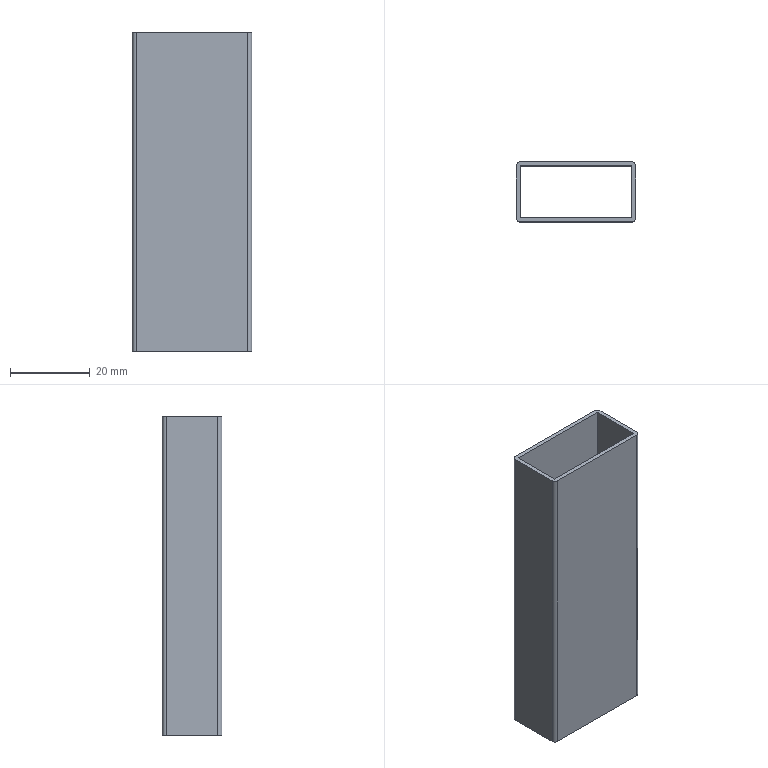Part | STEP file | Q7C1211 | 1 solid | 14 faces | box 30 x 15 x 80 mm | volume 6811 mm3 | plane 10 | cylinder 4 | commonest cylinder face diameters 2 x4
STEP:
#1=CARTESIAN_POINT('',(0.,0.,0.));
#2=DIRECTION('',(0.,0.,1.));
#3=DIRECTION('',(1.,0.,0.));
#4=AXIS2_PLACEMENT_3D('',#1,#2,#3);
#5=CARTESIAN_POINT('',(15.,6.5,40.));
#6=VERTEX_POINT('',#5);
#7=CARTESIAN_POINT('',(14.,7.5,40.));
#8=VERTEX_POINT('',#7);
#9=CARTESIAN_POINT('',(14.,6.5,40.));
#10=DIRECTION('',(0.,0.,1.));
#11=DIRECTION('',(-1.,0.,0.));
#12=AXIS2_PLACEMENT_3D('',#9,#10,#11);
#13=CIRCLE('',#12,1.);
#14=CARTESIAN_POINT('',(14.,6.5,40.));
#15=DIRECTION('',(0.,0.,-1.));
#16=DIRECTION('',(-1.,0.,0.));
#17=AXIS2_PLACEMENT_3D('',#14,#15,#16);
#18=PLANE('',#17);
#19=CARTESIAN_POINT('',(1.,0.));
#20=CARTESIAN_POINT('',(1.,-1.732));
#21=CARTESIAN_POINT('',(-0.5,-0.866));
#22=CARTESIAN_POINT('',(-2.,0.));
#23=CARTESIAN_POINT('',(-0.5,0.866));
#24=CARTESIAN_POINT('',(1.,1.732));
#25=CARTESIAN_POINT('',(1.,0.));
#26=(BOUNDED_CURVE()B_SPLINE_CURVE(2,(#19,#20,#21,#22,#23,#24,#25),.UNSPECIFIED.,.T.,.F.)B_SPLINE_CURVE_WITH_KNOTS((1,2,2,2,2,1),(-2.094,0.,2.094,4.189,6.283,8.378),.UNSPECIFIED.)CURVE()GEOMETRIC_REPRESENTATION_ITEM()RATIONAL_B_SPLINE_CURVE((1.,0.5,1.,0.5,1.,0.5,1.))REPRESENTATION_ITEM(''));
#27=(GEOMETRIC_REPRESENTATION_CONTEXT(2)PARAMETRIC_REPRESENTATION_CONTEXT()REPRESENTATION_CONTEXT('',''));
#28=DEFINITIONAL_REPRESENTATION('',(#26),#27);
#29=PCURVE('',#18,#28);
#30=CARTESIAN_POINT('',(14.,6.5,40.));
#31=DIRECTION('',(0.,0.,-1.));
#32=DIRECTION('',(-1.,0.,0.));
#33=AXIS2_PLACEMENT_3D('',#30,#31,#32);
#34=CYLINDRICAL_SURFACE('',#33,1.);
#35=CARTESIAN_POINT('',(6.283,0.));
#36=DIRECTION('',(-1.,0.));
#37=VECTOR('',#36,1.);
#38=LINE('',#35,#37);
#39=(GEOMETRIC_REPRESENTATION_CONTEXT(2)PARAMETRIC_REPRESENTATION_CONTEXT()REPRESENTATION_CONTEXT('',''));
#40=DEFINITIONAL_REPRESENTATION('',(#38),#39);
#41=PCURVE('',#34,#40);
#42=SURFACE_CURVE('',#13,(#29,#41),.PCURVE_S1.);
#43=EDGE_CURVE('',#6,#8,#42,.T.);
#44=ORIENTED_EDGE('',*,*,#43,.T.);
#45=CARTESIAN_POINT('',(-14.,7.5,40.));
#46=VERTEX_POINT('',#45);
#47=CARTESIAN_POINT('',(-14.,7.5,40.));
#48=DIRECTION('',(-1.,0.,0.));
#49=VECTOR('',#48,1.);
#50=LINE('',#47,#49);
#51=CARTESIAN_POINT('',(28.,1.));
#52=DIRECTION('',(1.,0.));
#53=VECTOR('',#52,1.);
#54=LINE('',#51,#53);
#55=(GEOMETRIC_REPRESENTATION_CONTEXT(2)PARAMETRIC_REPRESENTATION_CONTEXT()REPRESENTATION_CONTEXT('',''));
#56=DEFINITIONAL_REPRESENTATION('',(#54),#55);
#57=PCURVE('',#18,#56);
#58=CARTESIAN_POINT('',(-14.,7.5,40.));
#59=DIRECTION('',(0.,-1.,0.));
#60=DIRECTION('',(0.,0.,-1.));
#61=AXIS2_PLACEMENT_3D('',#58,#59,#60);
#62=PLANE('',#61);
#63=CARTESIAN_POINT('',(0.,0.));
#64=DIRECTION('',(0.,-1.));
#65=VECTOR('',#64,1.);
#66=LINE('',#63,#65);
#67=(GEOMETRIC_REPRESENTATION_CONTEXT(2)PARAMETRIC_REPRESENTATION_CONTEXT()REPRESENTATION_CONTEXT('',''));
#68=DEFINITIONAL_REPRESENTATION('',(#66),#67);
#69=PCURVE('',#62,#68);
#70=SURFACE_CURVE('',#50,(#57,#69),.PCURVE_S1.);
#71=EDGE_CURVE('',#8,#46,#70,.T.);
#72=ORIENTED_EDGE('',*,*,#71,.T.);
#73=CARTESIAN_POINT('',(-15.,6.5,40.));
#74=VERTEX_POINT('',#73);
#75=CARTESIAN_POINT('',(-14.,6.5,40.));
#76=DIRECTION('',(0.,0.,1.));
#77=DIRECTION('',(1.,0.,0.));
#78=AXIS2_PLACEMENT_3D('',#75,#76,#77);
#79=CIRCLE('',#78,1.);
#80=CARTESIAN_POINT('',(27.,0.));
#81=CARTESIAN_POINT('',(27.,1.732));
#82=CARTESIAN_POINT('',(28.5,0.866));
#83=CARTESIAN_POINT('',(30.,0.));
#84=CARTESIAN_POINT('',(28.5,-0.866));
#85=CARTESIAN_POINT('',(27.,-1.732));
#86=CARTESIAN_POINT('',(27.,0.));
#87=(BOUNDED_CURVE()B_SPLINE_CURVE(2,(#80,#81,#82,#83,#84,#85,#86),.UNSPECIFIED.,.T.,.F.)B_SPLINE_CURVE_WITH_KNOTS((1,2,2,2,2,1),(-2.094,0.,2.094,4.189,6.283,8.378),.UNSPECIFIED.)CURVE()GEOMETRIC_REPRESENTATION_ITEM()RATIONAL_B_SPLINE_CURVE((1.,0.5,1.,0.5,1.,0.5,1.))REPRESENTATION_ITEM(''));
#88=(GEOMETRIC_REPRESENTATION_CONTEXT(2)PARAMETRIC_REPRESENTATION_CONTEXT()REPRESENTATION_CONTEXT('',''));
#89=DEFINITIONAL_REPRESENTATION('',(#87),#88);
#90=PCURVE('',#18,#89);
#91=CARTESIAN_POINT('',(-14.,6.5,40.));
#92=DIRECTION('',(0.,0.,-1.));
#93=DIRECTION('',(-1.,0.,0.));
#94=AXIS2_PLACEMENT_3D('',#91,#92,#93);
#95=CYLINDRICAL_SURFACE('',#94,1.);
#96=CARTESIAN_POINT('',(3.142,0.));
#97=DIRECTION('',(-1.,0.));
#98=VECTOR('',#97,1.);
#99=LINE('',#96,#98);
#100=(GEOMETRIC_REPRESENTATION_CONTEXT(2)PARAMETRIC_REPRESENTATION_CONTEXT()REPRESENTATION_CONTEXT('',''));
#101=DEFINITIONAL_REPRESENTATION('',(#99),#100);
#102=PCURVE('',#95,#101);
#103=SURFACE_CURVE('',#79,(#90,#102),.PCURVE_S1.);
#104=EDGE_CURVE('',#46,#74,#103,.T.);
#105=ORIENTED_EDGE('',*,*,#104,.T.);
#106=CARTESIAN_POINT('',(-15.,-6.5,40.));
#107=VERTEX_POINT('',#106);
#108=CARTESIAN_POINT('',(-15.,6.5,40.));
#109=DIRECTION('',(0.,-1.,0.));
#110=VECTOR('',#109,1.);
#111=LINE('',#108,#110);
#112=CARTESIAN_POINT('',(29.,0.));
#113=DIRECTION('',(0.,-1.));
#114=VECTOR('',#113,1.);
#115=LINE('',#112,#114);
#116=(GEOMETRIC_REPRESENTATION_CONTEXT(2)PARAMETRIC_REPRESENTATION_CONTEXT()REPRESENTATION_CONTEXT('',''));
#117=DEFINITIONAL_REPRESENTATION('',(#115),#116);
#118=PCURVE('',#18,#117);
#119=CARTESIAN_POINT('',(-15.,6.5,40.));
#120=DIRECTION('',(1.,0.,0.));
#121=DIRECTION('',(0.,1.,0.));
#122=AXIS2_PLACEMENT_3D('',#119,#120,#121);
#123=PLANE('',#122);
#124=CARTESIAN_POINT('',(0.,0.));
#125=DIRECTION('',(-1.,0.));
#126=VECTOR('',#125,1.);
#127=LINE('',#124,#126);
#128=(GEOMETRIC_REPRESENTATION_CONTEXT(2)PARAMETRIC_REPRESENTATION_CONTEXT()REPRESENTATION_CONTEXT('',''));
#129=DEFINITIONAL_REPRESENTATION('',(#127),#128);
#130=PCURVE('',#123,#129);
#131=SURFACE_CURVE('',#111,(#118,#130),.PCURVE_S1.);
#132=EDGE_CURVE('',#74,#107,#131,.T.);
#133=ORIENTED_EDGE('',*,*,#132,.T.);
#134=CARTESIAN_POINT('',(-14.,-7.5,40.));
#135=VERTEX_POINT('',#134);
#136=CARTESIAN_POINT('',(-14.,-6.5,40.));
#137=DIRECTION('',(0.,0.,1.));
#138=DIRECTION('',(1.,0.,0.));
#139=AXIS2_PLACEMENT_3D('',#136,#137,#138);
#140=CIRCLE('',#139,1.);
#141=CARTESIAN_POINT('',(27.,-13.));
#142=CARTESIAN_POINT('',(27.,-11.268));
#143=CARTESIAN_POINT('',(28.5,-12.134));
#144=CARTESIAN_POINT('',(30.,-13.));
#145=CARTESIAN_POINT('',(28.5,-13.866));
#146=CARTESIAN_POINT('',(27.,-14.732));
#147=CARTESIAN_POINT('',(27.,-13.));
#148=(BOUNDED_CURVE()B_SPLINE_CURVE(2,(#141,#142,#143,#144,#145,#146,#147),.UNSPECIFIED.,.T.,.F.)B_SPLINE_CURVE_WITH_KNOTS((1,2,2,2,2,1),(-2.094,0.,2.094,4.189,6.283,8.378),.UNSPECIFIED.)CURVE()GEOMETRIC_REPRESENTATION_ITEM()RATIONAL_B_SPLINE_CURVE((1.,0.5,1.,0.5,1.,0.5,1.))REPRESENTATION_ITEM(''));
#149=(GEOMETRIC_REPRESENTATION_CONTEXT(2)PARAMETRIC_REPRESENTATION_CONTEXT()REPRESENTATION_CONTEXT('',''));
#150=DEFINITIONAL_REPRESENTATION('',(#148),#149);
#151=PCURVE('',#18,#150);
#152=CARTESIAN_POINT('',(-14.,-6.5,40.));
#153=DIRECTION('',(0.,0.,-1.));
#154=DIRECTION('',(-1.,0.,0.));
#155=AXIS2_PLACEMENT_3D('',#152,#153,#154);
#156=CYLINDRICAL_SURFACE('',#155,1.);
#157=CARTESIAN_POINT('',(9.425,0.));
#158=DIRECTION('',(-1.,0.));
#159=VECTOR('',#158,1.);
#160=LINE('',#157,#159);
#161=(GEOMETRIC_REPRESENTATION_CONTEXT(2)PARAMETRIC_REPRESENTATION_CONTEXT()REPRESENTATION_CONTEXT('',''));
#162=DEFINITIONAL_REPRESENTATION('',(#160),#161);
#163=PCURVE('',#156,#162);
#164=SURFACE_CURVE('',#140,(#151,#163),.PCURVE_S1.);
#165=EDGE_CURVE('',#107,#135,#164,.T.);
#166=ORIENTED_EDGE('',*,*,#165,.T.);
#167=CARTESIAN_POINT('',(14.,-7.5,40.));
#168=VERTEX_POINT('',#167);
#169=CARTESIAN_POINT('',(-14.,-7.5,40.));
#170=DIRECTION('',(1.,0.,0.));
#171=VECTOR('',#170,1.);
#172=LINE('',#169,#171);
#173=CARTESIAN_POINT('',(28.,-14.));
#174=DIRECTION('',(-1.,0.));
#175=VECTOR('',#174,1.);
#176=LINE('',#173,#175);
#177=(GEOMETRIC_REPRESENTATION_CONTEXT(2)PARAMETRIC_REPRESENTATION_CONTEXT()REPRESENTATION_CONTEXT('',''));
#178=DEFINITIONAL_REPRESENTATION('',(#176),#177);
#179=PCURVE('',#18,#178);
#180=CARTESIAN_POINT('',(-14.,-7.5,40.));
#181=DIRECTION('',(0.,1.,0.));
#182=DIRECTION('',(0.,0.,1.));
#183=AXIS2_PLACEMENT_3D('',#180,#181,#182);
#184=PLANE('',#183);
#185=CARTESIAN_POINT('',(0.,0.));
#186=DIRECTION('',(0.,1.));
#187=VECTOR('',#186,1.);
#188=LINE('',#185,#187);
#189=(GEOMETRIC_REPRESENTATION_CONTEXT(2)PARAMETRIC_REPRESENTATION_CONTEXT()REPRESENTATION_CONTEXT('',''));
#190=DEFINITIONAL_REPRESENTATION('',(#188),#189);
#191=PCURVE('',#184,#190);
#192=SURFACE_CURVE('',#172,(#179,#191),.PCURVE_S1.);
#193=EDGE_CURVE('',#135,#168,#192,.T.);
#194=ORIENTED_EDGE('',*,*,#193,.T.);
#195=CARTESIAN_POINT('',(15.,-6.5,40.));
#196=VERTEX_POINT('',#195);
#197=CARTESIAN_POINT('',(14.,-6.5,40.));
#198=DIRECTION('',(0.,0.,1.));
#199=DIRECTION('',(1.,0.,0.));
#200=AXIS2_PLACEMENT_3D('',#197,#198,#199);
#201=CIRCLE('',#200,1.);
#202=CARTESIAN_POINT('',(-1.,-13.));
#203=CARTESIAN_POINT('',(-1.,-11.268));
#204=CARTESIAN_POINT('',(0.5,-12.134));
#205=CARTESIAN_POINT('',(2.,-13.));
#206=CARTESIAN_POINT('',(0.5,-13.866));
#207=CARTESIAN_POINT('',(-1.,-14.732));
#208=CARTESIAN_POINT('',(-1.,-13.));
#209=(BOUNDED_CURVE()B_SPLINE_CURVE(2,(#202,#203,#204,#205,#206,#207,#208),.UNSPECIFIED.,.T.,.F.)B_SPLINE_CURVE_WITH_KNOTS((1,2,2,2,2,1),(-2.094,0.,2.094,4.189,6.283,8.378),.UNSPECIFIED.)CURVE()GEOMETRIC_REPRESENTATION_ITEM()RATIONAL_B_SPLINE_CURVE((1.,0.5,1.,0.5,1.,0.5,1.))REPRESENTATION_ITEM(''));
#210=(GEOMETRIC_REPRESENTATION_CONTEXT(2)PARAMETRIC_REPRESENTATION_CONTEXT()REPRESENTATION_CONTEXT('',''));
#211=DEFINITIONAL_REPRESENTATION('',(#209),#210);
#212=PCURVE('',#18,#211);
#213=CARTESIAN_POINT('',(14.,-6.5,40.));
#214=DIRECTION('',(0.,0.,-1.));
#215=DIRECTION('',(-1.,0.,0.));
#216=AXIS2_PLACEMENT_3D('',#213,#214,#215);
#217=CYLINDRICAL_SURFACE('',#216,1.);
#218=CARTESIAN_POINT('',(9.425,0.));
#219=DIRECTION('',(-1.,0.));
#220=VECTOR('',#219,1.);
#221=LINE('',#218,#220);
#222=(GEOMETRIC_REPRESENTATION_CONTEXT(2)PARAMETRIC_REPRESENTATION_CONTEXT()REPRESENTATION_CONTEXT('',''));
#223=DEFINITIONAL_REPRESENTATION('',(#221),#222);
#224=PCURVE('',#217,#223);
#225=SURFACE_CURVE('',#201,(#212,#224),.PCURVE_S1.);
#226=EDGE_CURVE('',#168,#196,#225,.T.);
#227=ORIENTED_EDGE('',*,*,#226,.T.);
#228=CARTESIAN_POINT('',(15.,6.5,40.));
#229=DIRECTION('',(0.,1.,0.));
#230=VECTOR('',#229,1.);
#231=LINE('',#228,#230);
#232=CARTESIAN_POINT('',(-1.,0.));
#233=DIRECTION('',(0.,1.));
#234=VECTOR('',#233,1.);
#235=LINE('',#232,#234);
#236=(GEOMETRIC_REPRESENTATION_CONTEXT(2)PARAMETRIC_REPRESENTATION_CONTEXT()REPRESENTATION_CONTEXT('',''));
#237=DEFINITIONAL_REPRESENTATION('',(#235),#236);
#238=PCURVE('',#18,#237);
#239=CARTESIAN_POINT('',(15.,6.5,40.));
#240=DIRECTION('',(-1.,0.,0.));
#241=DIRECTION('',(0.,0.,1.));
#242=AXIS2_PLACEMENT_3D('',#239,#240,#241);
#243=PLANE('',#242);
#244=CARTESIAN_POINT('',(0.,0.));
#245=DIRECTION('',(0.,1.));
#246=VECTOR('',#245,1.);
#247=LINE('',#244,#246);
#248=(GEOMETRIC_REPRESENTATION_CONTEXT(2)PARAMETRIC_REPRESENTATION_CONTEXT()REPRESENTATION_CONTEXT('',''));
#249=DEFINITIONAL_REPRESENTATION('',(#247),#248);
#250=PCURVE('',#243,#249);
#251=SURFACE_CURVE('',#231,(#238,#250),.PCURVE_S1.);
#252=EDGE_CURVE('',#196,#6,#251,.T.);
#253=ORIENTED_EDGE('',*,*,#252,.T.);
#254=EDGE_LOOP('',(#44,#72,#105,#133,#166,#194,#227,#253));
#255=FACE_BOUND('',#254,.T.);
#256=CARTESIAN_POINT('',(14.,6.5,40.));
#257=VERTEX_POINT('',#256);
#258=CARTESIAN_POINT('',(-14.,6.5,40.));
#259=VERTEX_POINT('',#258);
#260=CARTESIAN_POINT('',(-14.,6.5,40.));
#261=DIRECTION('',(-1.,0.,0.));
#262=VECTOR('',#261,1.);
#263=LINE('',#260,#262);
#264=CARTESIAN_POINT('',(28.,0.));
#265=DIRECTION('',(1.,0.));
#266=VECTOR('',#265,1.);
#267=LINE('',#264,#266);
#268=(GEOMETRIC_REPRESENTATION_CONTEXT(2)PARAMETRIC_REPRESENTATION_CONTEXT()REPRESENTATION_CONTEXT('',''));
#269=DEFINITIONAL_REPRESENTATION('',(#267),#268);
#270=PCURVE('',#18,#269);
#271=CARTESIAN_POINT('',(-14.,6.5,40.));
#272=DIRECTION('',(0.,-1.,0.));
#273=DIRECTION('',(0.,0.,-1.));
#274=AXIS2_PLACEMENT_3D('',#271,#272,#273);
#275=PLANE('',#274);
#276=CARTESIAN_POINT('',(0.,0.));
#277=DIRECTION('',(0.,-1.));
#278=VECTOR('',#277,1.);
#279=LINE('',#276,#278);
#280=(GEOMETRIC_REPRESENTATION_CONTEXT(2)PARAMETRIC_REPRESENTATION_CONTEXT()REPRESENTATION_CONTEXT('',''));
#281=DEFINITIONAL_REPRESENTATION('',(#279),#280);
#282=PCURVE('',#275,#281);
#283=SURFACE_CURVE('',#263,(#270,#282),.PCURVE_S1.);
#284=EDGE_CURVE('',#257,#259,#283,.T.);
#285=ORIENTED_EDGE('',*,*,#284,.F.);
#286=CARTESIAN_POINT('',(14.,-6.5,40.));
#287=VERTEX_POINT('',#286);
#288=CARTESIAN_POINT('',(14.,6.5,40.));
#289=DIRECTION('',(0.,1.,0.));
#290=VECTOR('',#289,1.);
#291=LINE('',#288,#290);
#292=CARTESIAN_POINT('',(0.,0.));
#293=DIRECTION('',(0.,1.));
#294=VECTOR('',#293,1.);
#295=LINE('',#292,#294);
#296=(GEOMETRIC_REPRESENTATION_CONTEXT(2)PARAMETRIC_REPRESENTATION_CONTEXT()REPRESENTATION_CONTEXT('',''));
#297=DEFINITIONAL_REPRESENTATION('',(#295),#296);
#298=PCURVE('',#18,#297);
#299=CARTESIAN_POINT('',(14.,6.5,40.));
#300=DIRECTION('',(-1.,0.,0.));
#301=DIRECTION('',(0.,-1.,0.));
#302=AXIS2_PLACEMENT_3D('',#299,#300,#301);
#303=PLANE('',#302);
#304=CARTESIAN_POINT('',(0.,0.));
#305=DIRECTION('',(-1.,0.));
#306=VECTOR('',#305,1.);
#307=LINE('',#304,#306);
#308=(GEOMETRIC_REPRESENTATION_CONTEXT(2)PARAMETRIC_REPRESENTATION_CONTEXT()REPRESENTATION_CONTEXT('',''));
#309=DEFINITIONAL_REPRESENTATION('',(#307),#308);
#310=PCURVE('',#303,#309);
#311=SURFACE_CURVE('',#291,(#298,#310),.PCURVE_S1.);
#312=EDGE_CURVE('',#287,#257,#311,.T.);
#313=ORIENTED_EDGE('',*,*,#312,.F.);
#314=CARTESIAN_POINT('',(-14.,-6.5,40.));
#315=VERTEX_POINT('',#314);
#316=CARTESIAN_POINT('',(-14.,-6.5,40.));
#317=DIRECTION('',(1.,0.,0.));
#318=VECTOR('',#317,1.);
#319=LINE('',#316,#318);
#320=CARTESIAN_POINT('',(28.,-13.));
#321=DIRECTION('',(-1.,0.));
#322=VECTOR('',#321,1.);
#323=LINE('',#320,#322);
#324=(GEOMETRIC_REPRESENTATION_CONTEXT(2)PARAMETRIC_REPRESENTATION_CONTEXT()REPRESENTATION_CONTEXT('',''));
#325=DEFINITIONAL_REPRESENTATION('',(#323),#324);
#326=PCURVE('',#18,#325);
#327=CARTESIAN_POINT('',(-14.,-6.5,40.));
#328=DIRECTION('',(0.,1.,0.));
#329=DIRECTION('',(0.,0.,1.));
#330=AXIS2_PLACEMENT_3D('',#327,#328,#329);
#331=PLANE('',#330);
#332=CARTESIAN_POINT('',(0.,0.));
#333=DIRECTION('',(0.,1.));
#334=VECTOR('',#333,1.);
#335=LINE('',#332,#334);
#336=(GEOMETRIC_REPRESENTATION_CONTEXT(2)PARAMETRIC_REPRESENTATION_CONTEXT()REPRESENTATION_CONTEXT('',''));
#337=DEFINITIONAL_REPRESENTATION('',(#335),#336);
#338=PCURVE('',#331,#337);
#339=SURFACE_CURVE('',#319,(#326,#338),.PCURVE_S1.);
#340=EDGE_CURVE('',#315,#287,#339,.T.);
#341=ORIENTED_EDGE('',*,*,#340,.F.);
#342=CARTESIAN_POINT('',(-14.,6.5,40.));
#343=DIRECTION('',(0.,-1.,0.));
#344=VECTOR('',#343,1.);
#345=LINE('',#342,#344);
#346=CARTESIAN_POINT('',(28.,0.));
#347=DIRECTION('',(0.,-1.));
#348=VECTOR('',#347,1.);
#349=LINE('',#346,#348);
#350=(GEOMETRIC_REPRESENTATION_CONTEXT(2)PARAMETRIC_REPRESENTATION_CONTEXT()REPRESENTATION_CONTEXT('',''));
#351=DEFINITIONAL_REPRESENTATION('',(#349),#350);
#352=PCURVE('',#18,#351);
#353=CARTESIAN_POINT('',(-14.,6.5,40.));
#354=DIRECTION('',(1.,0.,0.));
#355=DIRECTION('',(0.,1.,0.));
#356=AXIS2_PLACEMENT_3D('',#353,#354,#355);
#357=PLANE('',#356);
#358=CARTESIAN_POINT('',(0.,0.));
#359=DIRECTION('',(-1.,0.));
#360=VECTOR('',#359,1.);
#361=LINE('',#358,#360);
#362=(GEOMETRIC_REPRESENTATION_CONTEXT(2)PARAMETRIC_REPRESENTATION_CONTEXT()REPRESENTATION_CONTEXT('',''));
#363=DEFINITIONAL_REPRESENTATION('',(#361),#362);
#364=PCURVE('',#357,#363);
#365=SURFACE_CURVE('',#345,(#352,#364),.PCURVE_S1.);
#366=EDGE_CURVE('',#259,#315,#365,.T.);
#367=ORIENTED_EDGE('',*,*,#366,.F.);
#368=EDGE_LOOP('',(#285,#313,#341,#367));
#369=FACE_BOUND('',#368,.T.);
#370=ADVANCED_FACE('',(#255,#369),#18,.F.);
#371=CARTESIAN_POINT('',(15.,6.5,-40.));
#372=VERTEX_POINT('',#371);
#373=CARTESIAN_POINT('',(14.,7.5,-40.));
#374=VERTEX_POINT('',#373);
#375=CARTESIAN_POINT('',(14.,6.5,-40.));
#376=DIRECTION('',(0.,0.,1.));
#377=DIRECTION('',(-1.,0.,0.));
#378=AXIS2_PLACEMENT_3D('',#375,#376,#377);
#379=CIRCLE('',#378,1.);
#380=CARTESIAN_POINT('',(14.,6.5,-40.));
#381=DIRECTION('',(0.,0.,-1.));
#382=DIRECTION('',(-1.,0.,0.));
#383=AXIS2_PLACEMENT_3D('',#380,#381,#382);
#384=PLANE('',#383);
#385=CARTESIAN_POINT('',(1.,0.));
#386=CARTESIAN_POINT('',(1.,-1.732));
#387=CARTESIAN_POINT('',(-0.5,-0.866));
#388=CARTESIAN_POINT('',(-2.,0.));
#389=CARTESIAN_POINT('',(-0.5,0.866));
#390=CARTESIAN_POINT('',(1.,1.732));
#391=CARTESIAN_POINT('',(1.,0.));
#392=(BOUNDED_CURVE()B_SPLINE_CURVE(2,(#385,#386,#387,#388,#389,#390,#391),.UNSPECIFIED.,.T.,.F.)B_SPLINE_CURVE_WITH_KNOTS((1,2,2,2,2,1),(-2.094,0.,2.094,4.189,6.283,8.378),.UNSPECIFIED.)CURVE()GEOMETRIC_REPRESENTATION_ITEM()RATIONAL_B_SPLINE_CURVE((1.,0.5,1.,0.5,1.,0.5,1.))REPRESENTATION_ITEM(''));
#393=(GEOMETRIC_REPRESENTATION_CONTEXT(2)PARAMETRIC_REPRESENTATION_CONTEXT()REPRESENTATION_CONTEXT('',''));
#394=DEFINITIONAL_REPRESENTATION('',(#392),#393);
#395=PCURVE('',#384,#394);
#396=CARTESIAN_POINT('',(6.283,80.));
#397=DIRECTION('',(-1.,0.));
#398=VECTOR('',#397,1.);
#399=LINE('',#396,#398);
#400=(GEOMETRIC_REPRESENTATION_CONTEXT(2)PARAMETRIC_REPRESENTATION_CONTEXT()REPRESENTATION_CONTEXT('',''));
#401=DEFINITIONAL_REPRESENTATION('',(#399),#400);
#402=PCURVE('',#34,#401);
#403=SURFACE_CURVE('',#379,(#395,#402),.PCURVE_S1.);
#404=EDGE_CURVE('',#372,#374,#403,.T.);
#405=ORIENTED_EDGE('',*,*,#404,.F.);
#406=CARTESIAN_POINT('',(15.,-6.5,-40.));
#407=VERTEX_POINT('',#406);
#408=CARTESIAN_POINT('',(15.,6.5,-40.));
#409=DIRECTION('',(0.,1.,0.));
#410=VECTOR('',#409,1.);
#411=LINE('',#408,#410);
#412=CARTESIAN_POINT('',(-1.,0.));
#413=DIRECTION('',(0.,1.));
#414=VECTOR('',#413,1.);
#415=LINE('',#412,#414);
#416=(GEOMETRIC_REPRESENTATION_CONTEXT(2)PARAMETRIC_REPRESENTATION_CONTEXT()REPRESENTATION_CONTEXT('',''));
#417=DEFINITIONAL_REPRESENTATION('',(#415),#416);
#418=PCURVE('',#384,#417);
#419=CARTESIAN_POINT('',(-80.,0.));
#420=DIRECTION('',(0.,1.));
#421=VECTOR('',#420,1.);
#422=LINE('',#419,#421);
#423=(GEOMETRIC_REPRESENTATION_CONTEXT(2)PARAMETRIC_REPRESENTATION_CONTEXT()REPRESENTATION_CONTEXT('',''));
#424=DEFINITIONAL_REPRESENTATION('',(#422),#423);
#425=PCURVE('',#243,#424);
#426=SURFACE_CURVE('',#411,(#418,#425),.PCURVE_S1.);
#427=EDGE_CURVE('',#407,#372,#426,.T.);
#428=ORIENTED_EDGE('',*,*,#427,.F.);
#429=CARTESIAN_POINT('',(14.,-7.5,-40.));
#430=VERTEX_POINT('',#429);
#431=CARTESIAN_POINT('',(14.,-6.5,-40.));
#432=DIRECTION('',(0.,0.,1.));
#433=DIRECTION('',(1.,0.,0.));
#434=AXIS2_PLACEMENT_3D('',#431,#432,#433);
#435=CIRCLE('',#434,1.);
#436=CARTESIAN_POINT('',(-1.,-13.));
#437=CARTESIAN_POINT('',(-1.,-11.268));
#438=CARTESIAN_POINT('',(0.5,-12.134));
#439=CARTESIAN_POINT('',(2.,-13.));
#440=CARTESIAN_POINT('',(0.5,-13.866));
#441=CARTESIAN_POINT('',(-1.,-14.732));
#442=CARTESIAN_POINT('',(-1.,-13.));
#443=(BOUNDED_CURVE()B_SPLINE_CURVE(2,(#436,#437,#438,#439,#440,#441,#442),.UNSPECIFIED.,.T.,.F.)B_SPLINE_CURVE_WITH_KNOTS((1,2,2,2,2,1),(-2.094,0.,2.094,4.189,6.283,8.378),.UNSPECIFIED.)CURVE()GEOMETRIC_REPRESENTATION_ITEM()RATIONAL_B_SPLINE_CURVE((1.,0.5,1.,0.5,1.,0.5,1.))REPRESENTATION_ITEM(''));
#444=(GEOMETRIC_REPRESENTATION_CONTEXT(2)PARAMETRIC_REPRESENTATION_CONTEXT()REPRESENTATION_CONTEXT('',''));
#445=DEFINITIONAL_REPRESENTATION('',(#443),#444);
#446=PCURVE('',#384,#445);
#447=CARTESIAN_POINT('',(9.425,80.));
#448=DIRECTION('',(-1.,0.));
#449=VECTOR('',#448,1.);
#450=LINE('',#447,#449);
#451=(GEOMETRIC_REPRESENTATION_CONTEXT(2)PARAMETRIC_REPRESENTATION_CONTEXT()REPRESENTATION_CONTEXT('',''));
#452=DEFINITIONAL_REPRESENTATION('',(#450),#451);
#453=PCURVE('',#217,#452);
#454=SURFACE_CURVE('',#435,(#446,#453),.PCURVE_S1.);
#455=EDGE_CURVE('',#430,#407,#454,.T.);
#456=ORIENTED_EDGE('',*,*,#455,.F.);
#457=CARTESIAN_POINT('',(-14.,-7.5,-40.));
#458=VERTEX_POINT('',#457);
#459=CARTESIAN_POINT('',(-14.,-7.5,-40.));
#460=DIRECTION('',(1.,0.,0.));
#461=VECTOR('',#460,1.);
#462=LINE('',#459,#461);
#463=CARTESIAN_POINT('',(28.,-14.));
#464=DIRECTION('',(-1.,0.));
#465=VECTOR('',#464,1.);
#466=LINE('',#463,#465);
#467=(GEOMETRIC_REPRESENTATION_CONTEXT(2)PARAMETRIC_REPRESENTATION_CONTEXT()REPRESENTATION_CONTEXT('',''));
#468=DEFINITIONAL_REPRESENTATION('',(#466),#467);
#469=PCURVE('',#384,#468);
#470=CARTESIAN_POINT('',(-80.,0.));
#471=DIRECTION('',(0.,1.));
#472=VECTOR('',#471,1.);
#473=LINE('',#470,#472);
#474=(GEOMETRIC_REPRESENTATION_CONTEXT(2)PARAMETRIC_REPRESENTATION_CONTEXT()REPRESENTATION_CONTEXT('',''));
#475=DEFINITIONAL_REPRESENTATION('',(#473),#474);
#476=PCURVE('',#184,#475);
#477=SURFACE_CURVE('',#462,(#469,#476),.PCURVE_S1.);
#478=EDGE_CURVE('',#458,#430,#477,.T.);
#479=ORIENTED_EDGE('',*,*,#478,.F.);
#480=CARTESIAN_POINT('',(-15.,-6.5,-40.));
#481=VERTEX_POINT('',#480);
#482=CARTESIAN_POINT('',(-14.,-6.5,-40.));
#483=DIRECTION('',(0.,0.,1.));
#484=DIRECTION('',(1.,0.,0.));
#485=AXIS2_PLACEMENT_3D('',#482,#483,#484);
#486=CIRCLE('',#485,1.);
#487=CARTESIAN_POINT('',(27.,-13.));
#488=CARTESIAN_POINT('',(27.,-11.268));
#489=CARTESIAN_POINT('',(28.5,-12.134));
#490=CARTESIAN_POINT('',(30.,-13.));
#491=CARTESIAN_POINT('',(28.5,-13.866));
#492=CARTESIAN_POINT('',(27.,-14.732));
#493=CARTESIAN_POINT('',(27.,-13.));
#494=(BOUNDED_CURVE()B_SPLINE_CURVE(2,(#487,#488,#489,#490,#491,#492,#493),.UNSPECIFIED.,.T.,.F.)B_SPLINE_CURVE_WITH_KNOTS((1,2,2,2,2,1),(-2.094,0.,2.094,4.189,6.283,8.378),.UNSPECIFIED.)CURVE()GEOMETRIC_REPRESENTATION_ITEM()RATIONAL_B_SPLINE_CURVE((1.,0.5,1.,0.5,1.,0.5,1.))REPRESENTATION_ITEM(''));
#495=(GEOMETRIC_REPRESENTATION_CONTEXT(2)PARAMETRIC_REPRESENTATION_CONTEXT()REPRESENTATION_CONTEXT('',''));
#496=DEFINITIONAL_REPRESENTATION('',(#494),#495);
#497=PCURVE('',#384,#496);
#498=CARTESIAN_POINT('',(9.425,80.));
#499=DIRECTION('',(-1.,0.));
#500=VECTOR('',#499,1.);
#501=LINE('',#498,#500);
#502=(GEOMETRIC_REPRESENTATION_CONTEXT(2)PARAMETRIC_REPRESENTATION_CONTEXT()REPRESENTATION_CONTEXT('',''));
#503=DEFINITIONAL_REPRESENTATION('',(#501),#502);
#504=PCURVE('',#156,#503);
#505=SURFACE_CURVE('',#486,(#497,#504),.PCURVE_S1.);
#506=EDGE_CURVE('',#481,#458,#505,.T.);
#507=ORIENTED_EDGE('',*,*,#506,.F.);
#508=CARTESIAN_POINT('',(-15.,6.5,-40.));
#509=VERTEX_POINT('',#508);
#510=CARTESIAN_POINT('',(-15.,6.5,-40.));
#511=DIRECTION('',(0.,-1.,0.));
#512=VECTOR('',#511,1.);
#513=LINE('',#510,#512);
#514=CARTESIAN_POINT('',(29.,0.));
#515=DIRECTION('',(0.,-1.));
#516=VECTOR('',#515,1.);
#517=LINE('',#514,#516);
#518=(GEOMETRIC_REPRESENTATION_CONTEXT(2)PARAMETRIC_REPRESENTATION_CONTEXT()REPRESENTATION_CONTEXT('',''));
#519=DEFINITIONAL_REPRESENTATION('',(#517),#518);
#520=PCURVE('',#384,#519);
#521=CARTESIAN_POINT('',(0.,-80.));
#522=DIRECTION('',(-1.,0.));
#523=VECTOR('',#522,1.);
#524=LINE('',#521,#523);
#525=(GEOMETRIC_REPRESENTATION_CONTEXT(2)PARAMETRIC_REPRESENTATION_CONTEXT()REPRESENTATION_CONTEXT('',''));
#526=DEFINITIONAL_REPRESENTATION('',(#524),#525);
#527=PCURVE('',#123,#526);
#528=SURFACE_CURVE('',#513,(#520,#527),.PCURVE_S1.);
#529=EDGE_CURVE('',#509,#481,#528,.T.);
#530=ORIENTED_EDGE('',*,*,#529,.F.);
#531=CARTESIAN_POINT('',(-14.,7.5,-40.));
#532=VERTEX_POINT('',#531);
#533=CARTESIAN_POINT('',(-14.,6.5,-40.));
#534=DIRECTION('',(0.,0.,1.));
#535=DIRECTION('',(1.,0.,0.));
#536=AXIS2_PLACEMENT_3D('',#533,#534,#535);
#537=CIRCLE('',#536,1.);
#538=CARTESIAN_POINT('',(27.,0.));
#539=CARTESIAN_POINT('',(27.,1.732));
#540=CARTESIAN_POINT('',(28.5,0.866));
#541=CARTESIAN_POINT('',(30.,0.));
#542=CARTESIAN_POINT('',(28.5,-0.866));
#543=CARTESIAN_POINT('',(27.,-1.732));
#544=CARTESIAN_POINT('',(27.,0.));
#545=(BOUNDED_CURVE()B_SPLINE_CURVE(2,(#538,#539,#540,#541,#542,#543,#544),.UNSPECIFIED.,.T.,.F.)B_SPLINE_CURVE_WITH_KNOTS((1,2,2,2,2,1),(-2.094,0.,2.094,4.189,6.283,8.378),.UNSPECIFIED.)CURVE()GEOMETRIC_REPRESENTATION_ITEM()RATIONAL_B_SPLINE_CURVE((1.,0.5,1.,0.5,1.,0.5,1.))REPRESENTATION_ITEM(''));
#546=(GEOMETRIC_REPRESENTATION_CONTEXT(2)PARAMETRIC_REPRESENTATION_CONTEXT()REPRESENTATION_CONTEXT('',''));
#547=DEFINITIONAL_REPRESENTATION('',(#545),#546);
#548=PCURVE('',#384,#547);
#549=CARTESIAN_POINT('',(3.142,80.));
#550=DIRECTION('',(-1.,0.));
#551=VECTOR('',#550,1.);
#552=LINE('',#549,#551);
#553=(GEOMETRIC_REPRESENTATION_CONTEXT(2)PARAMETRIC_REPRESENTATION_CONTEXT()REPRESENTATION_CONTEXT('',''));
#554=DEFINITIONAL_REPRESENTATION('',(#552),#553);
#555=PCURVE('',#95,#554);
#556=SURFACE_CURVE('',#537,(#548,#555),.PCURVE_S1.);
#557=EDGE_CURVE('',#532,#509,#556,.T.);
#558=ORIENTED_EDGE('',*,*,#557,.F.);
#559=CARTESIAN_POINT('',(-14.,7.5,-40.));
#560=DIRECTION('',(-1.,0.,0.));
#561=VECTOR('',#560,1.);
#562=LINE('',#559,#561);
#563=CARTESIAN_POINT('',(28.,1.));
#564=DIRECTION('',(1.,0.));
#565=VECTOR('',#564,1.);
#566=LINE('',#563,#565);
#567=(GEOMETRIC_REPRESENTATION_CONTEXT(2)PARAMETRIC_REPRESENTATION_CONTEXT()REPRESENTATION_CONTEXT('',''));
#568=DEFINITIONAL_REPRESENTATION('',(#566),#567);
#569=PCURVE('',#384,#568);
#570=CARTESIAN_POINT('',(80.,0.));
#571=DIRECTION('',(0.,-1.));
#572=VECTOR('',#571,1.);
#573=LINE('',#570,#572);
#574=(GEOMETRIC_REPRESENTATION_CONTEXT(2)PARAMETRIC_REPRESENTATION_CONTEXT()REPRESENTATION_CONTEXT('',''));
#575=DEFINITIONAL_REPRESENTATION('',(#573),#574);
#576=PCURVE('',#62,#575);
#577=SURFACE_CURVE('',#562,(#569,#576),.PCURVE_S1.);
#578=EDGE_CURVE('',#374,#532,#577,.T.);
#579=ORIENTED_EDGE('',*,*,#578,.F.);
#580=EDGE_LOOP('',(#405,#428,#456,#479,#507,#530,#558,#579));
#581=FACE_BOUND('',#580,.T.);
#582=CARTESIAN_POINT('',(14.,-6.5,-40.));
#583=VERTEX_POINT('',#582);
#584=CARTESIAN_POINT('',(14.,6.5,-40.));
#585=VERTEX_POINT('',#584);
#586=CARTESIAN_POINT('',(14.,6.5,-40.));
#587=DIRECTION('',(0.,1.,0.));
#588=VECTOR('',#587,1.);
#589=LINE('',#586,#588);
#590=CARTESIAN_POINT('',(0.,0.));
#591=DIRECTION('',(0.,1.));
#592=VECTOR('',#591,1.);
#593=LINE('',#590,#592);
#594=(GEOMETRIC_REPRESENTATION_CONTEXT(2)PARAMETRIC_REPRESENTATION_CONTEXT()REPRESENTATION_CONTEXT('',''));
#595=DEFINITIONAL_REPRESENTATION('',(#593),#594);
#596=PCURVE('',#384,#595);
#597=CARTESIAN_POINT('',(0.,-80.));
#598=DIRECTION('',(-1.,0.));
#599=VECTOR('',#598,1.);
#600=LINE('',#597,#599);
#601=(GEOMETRIC_REPRESENTATION_CONTEXT(2)PARAMETRIC_REPRESENTATION_CONTEXT()REPRESENTATION_CONTEXT('',''));
#602=DEFINITIONAL_REPRESENTATION('',(#600),#601);
#603=PCURVE('',#303,#602);
#604=SURFACE_CURVE('',#589,(#596,#603),.PCURVE_S1.);
#605=EDGE_CURVE('',#583,#585,#604,.T.);
#606=ORIENTED_EDGE('',*,*,#605,.T.);
#607=CARTESIAN_POINT('',(-14.,6.5,-40.));
#608=VERTEX_POINT('',#607);
#609=CARTESIAN_POINT('',(-14.,6.5,-40.));
#610=DIRECTION('',(-1.,0.,0.));
#611=VECTOR('',#610,1.);
#612=LINE('',#609,#611);
#613=CARTESIAN_POINT('',(28.,0.));
#614=DIRECTION('',(1.,0.));
#615=VECTOR('',#614,1.);
#616=LINE('',#613,#615);
#617=(GEOMETRIC_REPRESENTATION_CONTEXT(2)PARAMETRIC_REPRESENTATION_CONTEXT()REPRESENTATION_CONTEXT('',''));
#618=DEFINITIONAL_REPRESENTATION('',(#616),#617);
#619=PCURVE('',#384,#618);
#620=CARTESIAN_POINT('',(80.,0.));
#621=DIRECTION('',(0.,-1.));
#622=VECTOR('',#621,1.);
#623=LINE('',#620,#622);
#624=(GEOMETRIC_REPRESENTATION_CONTEXT(2)PARAMETRIC_REPRESENTATION_CONTEXT()REPRESENTATION_CONTEXT('',''));
#625=DEFINITIONAL_REPRESENTATION('',(#623),#624);
#626=PCURVE('',#275,#625);
#627=SURFACE_CURVE('',#612,(#619,#626),.PCURVE_S1.);
#628=EDGE_CURVE('',#585,#608,#627,.T.);
#629=ORIENTED_EDGE('',*,*,#628,.T.);
#630=CARTESIAN_POINT('',(-14.,-6.5,-40.));
#631=VERTEX_POINT('',#630);
#632=CARTESIAN_POINT('',(-14.,6.5,-40.));
#633=DIRECTION('',(0.,-1.,0.));
#634=VECTOR('',#633,1.);
#635=LINE('',#632,#634);
#636=CARTESIAN_POINT('',(28.,0.));
#637=DIRECTION('',(0.,-1.));
#638=VECTOR('',#637,1.);
#639=LINE('',#636,#638);
#640=(GEOMETRIC_REPRESENTATION_CONTEXT(2)PARAMETRIC_REPRESENTATION_CONTEXT()REPRESENTATION_CONTEXT('',''));
#641=DEFINITIONAL_REPRESENTATION('',(#639),#640);
#642=PCURVE('',#384,#641);
#643=CARTESIAN_POINT('',(0.,-80.));
#644=DIRECTION('',(-1.,0.));
#645=VECTOR('',#644,1.);
#646=LINE('',#643,#645);
#647=(GEOMETRIC_REPRESENTATION_CONTEXT(2)PARAMETRIC_REPRESENTATION_CONTEXT()REPRESENTATION_CONTEXT('',''));
#648=DEFINITIONAL_REPRESENTATION('',(#646),#647);
#649=PCURVE('',#357,#648);
#650=SURFACE_CURVE('',#635,(#642,#649),.PCURVE_S1.);
#651=EDGE_CURVE('',#608,#631,#650,.T.);
#652=ORIENTED_EDGE('',*,*,#651,.T.);
#653=CARTESIAN_POINT('',(-14.,-6.5,-40.));
#654=DIRECTION('',(1.,0.,0.));
#655=VECTOR('',#654,1.);
#656=LINE('',#653,#655);
#657=CARTESIAN_POINT('',(28.,-13.));
#658=DIRECTION('',(-1.,0.));
#659=VECTOR('',#658,1.);
#660=LINE('',#657,#659);
#661=(GEOMETRIC_REPRESENTATION_CONTEXT(2)PARAMETRIC_REPRESENTATION_CONTEXT()REPRESENTATION_CONTEXT('',''));
#662=DEFINITIONAL_REPRESENTATION('',(#660),#661);
#663=PCURVE('',#384,#662);
#664=CARTESIAN_POINT('',(-80.,0.));
#665=DIRECTION('',(0.,1.));
#666=VECTOR('',#665,1.);
#667=LINE('',#664,#666);
#668=(GEOMETRIC_REPRESENTATION_CONTEXT(2)PARAMETRIC_REPRESENTATION_CONTEXT()REPRESENTATION_CONTEXT('',''));
#669=DEFINITIONAL_REPRESENTATION('',(#667),#668);
#670=PCURVE('',#331,#669);
#671=SURFACE_CURVE('',#656,(#663,#670),.PCURVE_S1.);
#672=EDGE_CURVE('',#631,#583,#671,.T.);
#673=ORIENTED_EDGE('',*,*,#672,.T.);
#674=EDGE_LOOP('',(#606,#629,#652,#673));
#675=FACE_BOUND('',#674,.T.);
#676=ADVANCED_FACE('',(#581,#675),#384,.T.);
#677=ORIENTED_EDGE('',*,*,#404,.T.);
#678=CARTESIAN_POINT('',(14.,7.5,40.));
#679=DIRECTION('',(0.,0.,-1.));
#680=VECTOR('',#679,1.);
#681=LINE('',#678,#680);
#682=CARTESIAN_POINT('',(1.571,0.));
#683=DIRECTION('',(0.,1.));
#684=VECTOR('',#683,1.);
#685=LINE('',#682,#684);
#686=(GEOMETRIC_REPRESENTATION_CONTEXT(2)PARAMETRIC_REPRESENTATION_CONTEXT()REPRESENTATION_CONTEXT('',''));
#687=DEFINITIONAL_REPRESENTATION('',(#685),#686);
#688=PCURVE('',#34,#687);
#689=CARTESIAN_POINT('',(0.,28.));
#690=DIRECTION('',(1.,0.));
#691=VECTOR('',#690,1.);
#692=LINE('',#689,#691);
#693=(GEOMETRIC_REPRESENTATION_CONTEXT(2)PARAMETRIC_REPRESENTATION_CONTEXT()REPRESENTATION_CONTEXT('',''));
#694=DEFINITIONAL_REPRESENTATION('',(#692),#693);
#695=PCURVE('',#62,#694);
#696=SURFACE_CURVE('',#681,(#688,#695),.PCURVE_S1.);
#697=EDGE_CURVE('',#8,#374,#696,.T.);
#698=ORIENTED_EDGE('',*,*,#697,.F.);
#699=ORIENTED_EDGE('',*,*,#43,.F.);
#700=CARTESIAN_POINT('',(15.,6.5,40.));
#701=DIRECTION('',(0.,0.,-1.));
#702=VECTOR('',#701,1.);
#703=LINE('',#700,#702);
#704=CARTESIAN_POINT('',(3.142,0.));
#705=DIRECTION('',(0.,1.));
#706=VECTOR('',#705,1.);
#707=LINE('',#704,#706);
#708=(GEOMETRIC_REPRESENTATION_CONTEXT(2)PARAMETRIC_REPRESENTATION_CONTEXT()REPRESENTATION_CONTEXT('',''));
#709=DEFINITIONAL_REPRESENTATION('',(#707),#708);
#710=PCURVE('',#34,#709);
#711=CARTESIAN_POINT('',(0.,0.));
#712=DIRECTION('',(-1.,0.));
#713=VECTOR('',#712,1.);
#714=LINE('',#711,#713);
#715=(GEOMETRIC_REPRESENTATION_CONTEXT(2)PARAMETRIC_REPRESENTATION_CONTEXT()REPRESENTATION_CONTEXT('',''));
#716=DEFINITIONAL_REPRESENTATION('',(#714),#715);
#717=PCURVE('',#243,#716);
#718=SURFACE_CURVE('',#703,(#710,#717),.PCURVE_S1.);
#719=EDGE_CURVE('',#6,#372,#718,.T.);
#720=ORIENTED_EDGE('',*,*,#719,.T.);
#721=EDGE_LOOP('',(#677,#698,#699,#720));
#722=FACE_BOUND('',#721,.T.);
#723=ADVANCED_FACE('',(#722),#34,.T.);
#724=ORIENTED_EDGE('',*,*,#578,.T.);
#725=CARTESIAN_POINT('',(-14.,7.5,40.));
#726=DIRECTION('',(0.,0.,-1.));
#727=VECTOR('',#726,1.);
#728=LINE('',#725,#727);
#729=CARTESIAN_POINT('',(0.,0.));
#730=DIRECTION('',(1.,0.));
#731=VECTOR('',#730,1.);
#732=LINE('',#729,#731);
#733=(GEOMETRIC_REPRESENTATION_CONTEXT(2)PARAMETRIC_REPRESENTATION_CONTEXT()REPRESENTATION_CONTEXT('',''));
#734=DEFINITIONAL_REPRESENTATION('',(#732),#733);
#735=PCURVE('',#62,#734);
#736=CARTESIAN_POINT('',(1.571,0.));
#737=DIRECTION('',(0.,1.));
#738=VECTOR('',#737,1.);
#739=LINE('',#736,#738);
#740=(GEOMETRIC_REPRESENTATION_CONTEXT(2)PARAMETRIC_REPRESENTATION_CONTEXT()REPRESENTATION_CONTEXT('',''));
#741=DEFINITIONAL_REPRESENTATION('',(#739),#740);
#742=PCURVE('',#95,#741);
#743=SURFACE_CURVE('',#728,(#735,#742),.PCURVE_S1.);
#744=EDGE_CURVE('',#46,#532,#743,.T.);
#745=ORIENTED_EDGE('',*,*,#744,.F.);
#746=ORIENTED_EDGE('',*,*,#71,.F.);
#747=ORIENTED_EDGE('',*,*,#697,.T.);
#748=EDGE_LOOP('',(#724,#745,#746,#747));
#749=FACE_BOUND('',#748,.T.);
#750=ADVANCED_FACE('',(#749),#62,.F.);
#751=ORIENTED_EDGE('',*,*,#557,.T.);
#752=CARTESIAN_POINT('',(-15.,6.5,40.));
#753=DIRECTION('',(0.,0.,-1.));
#754=VECTOR('',#753,1.);
#755=LINE('',#752,#754);
#756=CARTESIAN_POINT('',(0.,0.));
#757=DIRECTION('',(0.,1.));
#758=VECTOR('',#757,1.);
#759=LINE('',#756,#758);
#760=(GEOMETRIC_REPRESENTATION_CONTEXT(2)PARAMETRIC_REPRESENTATION_CONTEXT()REPRESENTATION_CONTEXT('',''));
#761=DEFINITIONAL_REPRESENTATION('',(#759),#760);
#762=PCURVE('',#95,#761);
#763=CARTESIAN_POINT('',(0.,0.));
#764=DIRECTION('',(0.,-1.));
#765=VECTOR('',#764,1.);
#766=LINE('',#763,#765);
#767=(GEOMETRIC_REPRESENTATION_CONTEXT(2)PARAMETRIC_REPRESENTATION_CONTEXT()REPRESENTATION_CONTEXT('',''));
#768=DEFINITIONAL_REPRESENTATION('',(#766),#767);
#769=PCURVE('',#123,#768);
#770=SURFACE_CURVE('',#755,(#762,#769),.PCURVE_S1.);
#771=EDGE_CURVE('',#74,#509,#770,.T.);
#772=ORIENTED_EDGE('',*,*,#771,.F.);
#773=ORIENTED_EDGE('',*,*,#104,.F.);
#774=ORIENTED_EDGE('',*,*,#744,.T.);
#775=EDGE_LOOP('',(#751,#772,#773,#774));
#776=FACE_BOUND('',#775,.T.);
#777=ADVANCED_FACE('',(#776),#95,.T.);
#778=ORIENTED_EDGE('',*,*,#529,.T.);
#779=CARTESIAN_POINT('',(-15.,-6.5,40.));
#780=DIRECTION('',(0.,0.,-1.));
#781=VECTOR('',#780,1.);
#782=LINE('',#779,#781);
#783=CARTESIAN_POINT('',(-13.,0.));
#784=DIRECTION('',(0.,-1.));
#785=VECTOR('',#784,1.);
#786=LINE('',#783,#785);
#787=(GEOMETRIC_REPRESENTATION_CONTEXT(2)PARAMETRIC_REPRESENTATION_CONTEXT()REPRESENTATION_CONTEXT('',''));
#788=DEFINITIONAL_REPRESENTATION('',(#786),#787);
#789=PCURVE('',#123,#788);
#790=CARTESIAN_POINT('',(6.283,0.));
#791=DIRECTION('',(0.,1.));
#792=VECTOR('',#791,1.);
#793=LINE('',#790,#792);
#794=(GEOMETRIC_REPRESENTATION_CONTEXT(2)PARAMETRIC_REPRESENTATION_CONTEXT()REPRESENTATION_CONTEXT('',''));
#795=DEFINITIONAL_REPRESENTATION('',(#793),#794);
#796=PCURVE('',#156,#795);
#797=SURFACE_CURVE('',#782,(#789,#796),.PCURVE_S1.);
#798=EDGE_CURVE('',#107,#481,#797,.T.);
#799=ORIENTED_EDGE('',*,*,#798,.F.);
#800=ORIENTED_EDGE('',*,*,#132,.F.);
#801=ORIENTED_EDGE('',*,*,#771,.T.);
#802=EDGE_LOOP('',(#778,#799,#800,#801));
#803=FACE_BOUND('',#802,.T.);
#804=ADVANCED_FACE('',(#803),#123,.F.);
#805=ORIENTED_EDGE('',*,*,#506,.T.);
#806=CARTESIAN_POINT('',(-14.,-7.5,40.));
#807=DIRECTION('',(0.,0.,-1.));
#808=VECTOR('',#807,1.);
#809=LINE('',#806,#808);
#810=CARTESIAN_POINT('',(4.712,0.));
#811=DIRECTION('',(0.,1.));
#812=VECTOR('',#811,1.);
#813=LINE('',#810,#812);
#814=(GEOMETRIC_REPRESENTATION_CONTEXT(2)PARAMETRIC_REPRESENTATION_CONTEXT()REPRESENTATION_CONTEXT('',''));
#815=DEFINITIONAL_REPRESENTATION('',(#813),#814);
#816=PCURVE('',#156,#815);
#817=CARTESIAN_POINT('',(0.,0.));
#818=DIRECTION('',(-1.,0.));
#819=VECTOR('',#818,1.);
#820=LINE('',#817,#819);
#821=(GEOMETRIC_REPRESENTATION_CONTEXT(2)PARAMETRIC_REPRESENTATION_CONTEXT()REPRESENTATION_CONTEXT('',''));
#822=DEFINITIONAL_REPRESENTATION('',(#820),#821);
#823=PCURVE('',#184,#822);
#824=SURFACE_CURVE('',#809,(#816,#823),.PCURVE_S1.);
#825=EDGE_CURVE('',#135,#458,#824,.T.);
#826=ORIENTED_EDGE('',*,*,#825,.F.);
#827=ORIENTED_EDGE('',*,*,#165,.F.);
#828=ORIENTED_EDGE('',*,*,#798,.T.);
#829=EDGE_LOOP('',(#805,#826,#827,#828));
#830=FACE_BOUND('',#829,.T.);
#831=ADVANCED_FACE('',(#830),#156,.T.);
#832=ORIENTED_EDGE('',*,*,#478,.T.);
#833=CARTESIAN_POINT('',(14.,-7.5,40.));
#834=DIRECTION('',(0.,0.,-1.));
#835=VECTOR('',#834,1.);
#836=LINE('',#833,#835);
#837=CARTESIAN_POINT('',(0.,28.));
#838=DIRECTION('',(-1.,0.));
#839=VECTOR('',#838,1.);
#840=LINE('',#837,#839);
#841=(GEOMETRIC_REPRESENTATION_CONTEXT(2)PARAMETRIC_REPRESENTATION_CONTEXT()REPRESENTATION_CONTEXT('',''));
#842=DEFINITIONAL_REPRESENTATION('',(#840),#841);
#843=PCURVE('',#184,#842);
#844=CARTESIAN_POINT('',(4.712,0.));
#845=DIRECTION('',(0.,1.));
#846=VECTOR('',#845,1.);
#847=LINE('',#844,#846);
#848=(GEOMETRIC_REPRESENTATION_CONTEXT(2)PARAMETRIC_REPRESENTATION_CONTEXT()REPRESENTATION_CONTEXT('',''));
#849=DEFINITIONAL_REPRESENTATION('',(#847),#848);
#850=PCURVE('',#217,#849);
#851=SURFACE_CURVE('',#836,(#843,#850),.PCURVE_S1.);
#852=EDGE_CURVE('',#168,#430,#851,.T.);
#853=ORIENTED_EDGE('',*,*,#852,.F.);
#854=ORIENTED_EDGE('',*,*,#193,.F.);
#855=ORIENTED_EDGE('',*,*,#825,.T.);
#856=EDGE_LOOP('',(#832,#853,#854,#855));
#857=FACE_BOUND('',#856,.T.);
#858=ADVANCED_FACE('',(#857),#184,.F.);
#859=ORIENTED_EDGE('',*,*,#455,.T.);
#860=CARTESIAN_POINT('',(15.,-6.5,40.));
#861=DIRECTION('',(0.,0.,-1.));
#862=VECTOR('',#861,1.);
#863=LINE('',#860,#862);
#864=CARTESIAN_POINT('',(3.142,0.));
#865=DIRECTION('',(0.,1.));
#866=VECTOR('',#865,1.);
#867=LINE('',#864,#866);
#868=(GEOMETRIC_REPRESENTATION_CONTEXT(2)PARAMETRIC_REPRESENTATION_CONTEXT()REPRESENTATION_CONTEXT('',''));
#869=DEFINITIONAL_REPRESENTATION('',(#867),#868);
#870=PCURVE('',#217,#869);
#871=CARTESIAN_POINT('',(0.,-13.));
#872=DIRECTION('',(-1.,0.));
#873=VECTOR('',#872,1.);
#874=LINE('',#871,#873);
#875=(GEOMETRIC_REPRESENTATION_CONTEXT(2)PARAMETRIC_REPRESENTATION_CONTEXT()REPRESENTATION_CONTEXT('',''));
#876=DEFINITIONAL_REPRESENTATION('',(#874),#875);
#877=PCURVE('',#243,#876);
#878=SURFACE_CURVE('',#863,(#870,#877),.PCURVE_S1.);
#879=EDGE_CURVE('',#196,#407,#878,.T.);
#880=ORIENTED_EDGE('',*,*,#879,.F.);
#881=ORIENTED_EDGE('',*,*,#226,.F.);
#882=ORIENTED_EDGE('',*,*,#852,.T.);
#883=EDGE_LOOP('',(#859,#880,#881,#882));
#884=FACE_BOUND('',#883,.T.);
#885=ADVANCED_FACE('',(#884),#217,.T.);
#886=ORIENTED_EDGE('',*,*,#427,.T.);
#887=ORIENTED_EDGE('',*,*,#719,.F.);
#888=ORIENTED_EDGE('',*,*,#252,.F.);
#889=ORIENTED_EDGE('',*,*,#879,.T.);
#890=EDGE_LOOP('',(#886,#887,#888,#889));
#891=FACE_BOUND('',#890,.T.);
#892=ADVANCED_FACE('',(#891),#243,.F.);
#893=ORIENTED_EDGE('',*,*,#628,.F.);
#894=CARTESIAN_POINT('',(14.,6.5,40.));
#895=DIRECTION('',(0.,0.,-1.));
#896=VECTOR('',#895,1.);
#897=LINE('',#894,#896);
#898=CARTESIAN_POINT('',(0.,28.));
#899=DIRECTION('',(1.,0.));
#900=VECTOR('',#899,1.);
#901=LINE('',#898,#900);
#902=(GEOMETRIC_REPRESENTATION_CONTEXT(2)PARAMETRIC_REPRESENTATION_CONTEXT()REPRESENTATION_CONTEXT('',''));
#903=DEFINITIONAL_REPRESENTATION('',(#901),#902);
#904=PCURVE('',#275,#903);
#905=CARTESIAN_POINT('',(0.,0.));
#906=DIRECTION('',(0.,-1.));
#907=VECTOR('',#906,1.);
#908=LINE('',#905,#907);
#909=(GEOMETRIC_REPRESENTATION_CONTEXT(2)PARAMETRIC_REPRESENTATION_CONTEXT()REPRESENTATION_CONTEXT('',''));
#910=DEFINITIONAL_REPRESENTATION('',(#908),#909);
#911=PCURVE('',#303,#910);
#912=SURFACE_CURVE('',#897,(#904,#911),.PCURVE_S1.);
#913=EDGE_CURVE('',#257,#585,#912,.T.);
#914=ORIENTED_EDGE('',*,*,#913,.F.);
#915=ORIENTED_EDGE('',*,*,#284,.T.);
#916=CARTESIAN_POINT('',(-14.,6.5,40.));
#917=DIRECTION('',(0.,0.,-1.));
#918=VECTOR('',#917,1.);
#919=LINE('',#916,#918);
#920=CARTESIAN_POINT('',(0.,0.));
#921=DIRECTION('',(1.,0.));
#922=VECTOR('',#921,1.);
#923=LINE('',#920,#922);
#924=(GEOMETRIC_REPRESENTATION_CONTEXT(2)PARAMETRIC_REPRESENTATION_CONTEXT()REPRESENTATION_CONTEXT('',''));
#925=DEFINITIONAL_REPRESENTATION('',(#923),#924);
#926=PCURVE('',#275,#925);
#927=CARTESIAN_POINT('',(0.,0.));
#928=DIRECTION('',(0.,-1.));
#929=VECTOR('',#928,1.);
#930=LINE('',#927,#929);
#931=(GEOMETRIC_REPRESENTATION_CONTEXT(2)PARAMETRIC_REPRESENTATION_CONTEXT()REPRESENTATION_CONTEXT('',''));
#932=DEFINITIONAL_REPRESENTATION('',(#930),#931);
#933=PCURVE('',#357,#932);
#934=SURFACE_CURVE('',#919,(#926,#933),.PCURVE_S1.);
#935=EDGE_CURVE('',#259,#608,#934,.T.);
#936=ORIENTED_EDGE('',*,*,#935,.T.);
#937=EDGE_LOOP('',(#893,#914,#915,#936));
#938=FACE_BOUND('',#937,.T.);
#939=ADVANCED_FACE('',(#938),#275,.T.);
#940=ORIENTED_EDGE('',*,*,#651,.F.);
#941=ORIENTED_EDGE('',*,*,#935,.F.);
#942=ORIENTED_EDGE('',*,*,#366,.T.);
#943=CARTESIAN_POINT('',(-14.,-6.5,40.));
#944=DIRECTION('',(0.,0.,-1.));
#945=VECTOR('',#944,1.);
#946=LINE('',#943,#945);
#947=CARTESIAN_POINT('',(-13.,0.));
#948=DIRECTION('',(0.,-1.));
#949=VECTOR('',#948,1.);
#950=LINE('',#947,#949);
#951=(GEOMETRIC_REPRESENTATION_CONTEXT(2)PARAMETRIC_REPRESENTATION_CONTEXT()REPRESENTATION_CONTEXT('',''));
#952=DEFINITIONAL_REPRESENTATION('',(#950),#951);
#953=PCURVE('',#357,#952);
#954=CARTESIAN_POINT('',(0.,0.));
#955=DIRECTION('',(-1.,0.));
#956=VECTOR('',#955,1.);
#957=LINE('',#954,#956);
#958=(GEOMETRIC_REPRESENTATION_CONTEXT(2)PARAMETRIC_REPRESENTATION_CONTEXT()REPRESENTATION_CONTEXT('',''));
#959=DEFINITIONAL_REPRESENTATION('',(#957),#958);
#960=PCURVE('',#331,#959);
#961=SURFACE_CURVE('',#946,(#953,#960),.PCURVE_S1.);
#962=EDGE_CURVE('',#315,#631,#961,.T.);
#963=ORIENTED_EDGE('',*,*,#962,.T.);
#964=EDGE_LOOP('',(#940,#941,#942,#963));
#965=FACE_BOUND('',#964,.T.);
#966=ADVANCED_FACE('',(#965),#357,.T.);
#967=ORIENTED_EDGE('',*,*,#672,.F.);
#968=ORIENTED_EDGE('',*,*,#962,.F.);
#969=ORIENTED_EDGE('',*,*,#340,.T.);
#970=CARTESIAN_POINT('',(14.,-6.5,40.));
#971=DIRECTION('',(0.,0.,-1.));
#972=VECTOR('',#971,1.);
#973=LINE('',#970,#972);
#974=CARTESIAN_POINT('',(0.,28.));
#975=DIRECTION('',(-1.,0.));
#976=VECTOR('',#975,1.);
#977=LINE('',#974,#976);
#978=(GEOMETRIC_REPRESENTATION_CONTEXT(2)PARAMETRIC_REPRESENTATION_CONTEXT()REPRESENTATION_CONTEXT('',''));
#979=DEFINITIONAL_REPRESENTATION('',(#977),#978);
#980=PCURVE('',#331,#979);
#981=CARTESIAN_POINT('',(13.,0.));
#982=DIRECTION('',(0.,-1.));
#983=VECTOR('',#982,1.);
#984=LINE('',#981,#983);
#985=(GEOMETRIC_REPRESENTATION_CONTEXT(2)PARAMETRIC_REPRESENTATION_CONTEXT()REPRESENTATION_CONTEXT('',''));
#986=DEFINITIONAL_REPRESENTATION('',(#984),#985);
#987=PCURVE('',#303,#986);
#988=SURFACE_CURVE('',#973,(#980,#987),.PCURVE_S1.);
#989=EDGE_CURVE('',#287,#583,#988,.T.);
#990=ORIENTED_EDGE('',*,*,#989,.T.);
#991=EDGE_LOOP('',(#967,#968,#969,#990));
#992=FACE_BOUND('',#991,.T.);
#993=ADVANCED_FACE('',(#992),#331,.T.);
#994=ORIENTED_EDGE('',*,*,#605,.F.);
#995=ORIENTED_EDGE('',*,*,#989,.F.);
#996=ORIENTED_EDGE('',*,*,#312,.T.);
#997=ORIENTED_EDGE('',*,*,#913,.T.);
#998=EDGE_LOOP('',(#994,#995,#996,#997));
#999=FACE_BOUND('',#998,.T.);
#1000=ADVANCED_FACE('',(#999),#303,.T.);
#1001=CLOSED_SHELL('',(#370,#676,#723,#750,#777,#804,#831,#858,#885,#892,#939,#966,#993,#1000));
#1002=MANIFOLD_SOLID_BREP('',#1001);
#1003=(LENGTH_UNIT()NAMED_UNIT(*)SI_UNIT(.MILLI.,.METRE.));
#1004=UNCERTAINTY_MEASURE_WITH_UNIT(LENGTH_MEASURE(0.0000001),#1003,'','');
#1005=(NAMED_UNIT(*)PLANE_ANGLE_UNIT()SI_UNIT($,.RADIAN.));
#1006=(NAMED_UNIT(*)SI_UNIT($,.STERADIAN.)SOLID_ANGLE_UNIT());
#1007=(GEOMETRIC_REPRESENTATION_CONTEXT(3)GLOBAL_UNCERTAINTY_ASSIGNED_CONTEXT((#1004))GLOBAL_UNIT_ASSIGNED_CONTEXT((#1003,#1005,#1006))REPRESENTATION_CONTEXT('',''));
#1008=ADVANCED_BREP_SHAPE_REPRESENTATION('',(#4,#1002),#1007);